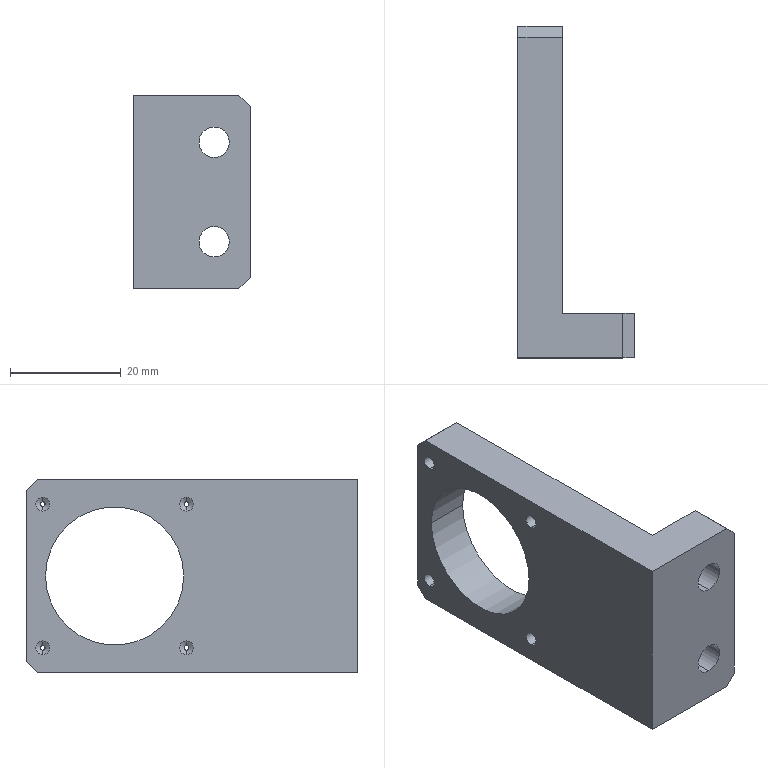Part | NX | features BREP 1 | 1 solid | 34 faces | box 21 x 60 x 35 mm | volume 15917 mm3 | cylinder 14 | plane 12 | cone 8 | commonest cylinder face diameters 2.5 x8 5.5 x4 25 x2
STEP:
#1=CARTESIAN_POINT('',(3.227,27.193,17.5));
#2=VERTEX_POINT('',#1);
#3=CARTESIAN_POINT('',(3.227,2.193,17.5));
#4=VERTEX_POINT('',#3);
#5=CARTESIAN_POINT('',(3.227,14.693,17.5));
#6=DIRECTION('',(-1.,0.,0.));
#7=DIRECTION('',(0.,1.,0.));
#8=AXIS2_PLACEMENT_3D('',#5,#6,#7);
#9=CIRCLE('',#8,12.5);
#10=EDGE_CURVE('',#2,#4,#9,.T.);
#11=ORIENTED_EDGE('',*,*,#10,.T.);
#12=CARTESIAN_POINT('',(11.227,2.193,17.5));
#13=VERTEX_POINT('',#12);
#14=CARTESIAN_POINT('',(3.227,2.193,17.5));
#15=DIRECTION('',(1.,0.,0.));
#16=VECTOR('',#15,1000.);
#17=LINE('',#14,#16);
#18=EDGE_CURVE('',#13,#4,#17,.F.);
#19=ORIENTED_EDGE('',*,*,#18,.F.);
#20=CARTESIAN_POINT('',(11.227,27.193,17.5));
#21=VERTEX_POINT('',#20);
#22=CARTESIAN_POINT('',(11.227,14.693,17.5));
#23=DIRECTION('',(-1.,0.,0.));
#24=DIRECTION('',(0.,1.,0.));
#25=AXIS2_PLACEMENT_3D('',#22,#23,#24);
#26=CIRCLE('',#25,12.5);
#27=EDGE_CURVE('',#21,#13,#26,.T.);
#28=ORIENTED_EDGE('',*,*,#27,.F.);
#29=CARTESIAN_POINT('',(3.227,27.193,17.5));
#30=DIRECTION('',(1.,0.,0.));
#31=VECTOR('',#30,1000.);
#32=LINE('',#29,#31);
#33=EDGE_CURVE('',#21,#2,#32,.F.);
#34=ORIENTED_EDGE('',*,*,#33,.T.);
#35=EDGE_LOOP('',(#11,#19,#28,#34));
#36=FACE_BOUND('',#35,.T.);
#37=CARTESIAN_POINT('',(3.227,14.693,17.5));
#38=DIRECTION('',(1.,0.,0.));
#39=DIRECTION('',(0.,1.,0.));
#40=AXIS2_PLACEMENT_3D('',#37,#38,#39);
#41=CYLINDRICAL_SURFACE('',#40,12.5);
#42=ADVANCED_FACE('',(#36),#41,.F.);
#43=CARTESIAN_POINT('',(10.727,1.693,3.25));
#44=VERTEX_POINT('',#43);
#45=CARTESIAN_POINT('',(10.727,1.693,5.75));
#46=VERTEX_POINT('',#45);
#47=CARTESIAN_POINT('',(10.727,1.693,4.5));
#48=DIRECTION('',(-1.,0.,0.));
#49=DIRECTION('',(0.,0.,1.));
#50=AXIS2_PLACEMENT_3D('',#47,#48,#49);
#51=CIRCLE('',#50,1.25);
#52=EDGE_CURVE('',#44,#46,#51,.T.);
#53=ORIENTED_EDGE('',*,*,#52,.F.);
#54=CARTESIAN_POINT('',(3.227,1.693,3.25));
#55=VERTEX_POINT('',#54);
#56=CARTESIAN_POINT('',(3.227,1.693,3.25));
#57=DIRECTION('',(-1.,0.,0.));
#58=VECTOR('',#57,1000.);
#59=LINE('',#56,#58);
#60=EDGE_CURVE('',#55,#44,#59,.F.);
#61=ORIENTED_EDGE('',*,*,#60,.F.);
#62=CARTESIAN_POINT('',(3.227,1.693,5.75));
#63=VERTEX_POINT('',#62);
#64=CARTESIAN_POINT('',(3.227,1.693,4.5));
#65=DIRECTION('',(-1.,0.,0.));
#66=DIRECTION('',(0.,0.,1.));
#67=AXIS2_PLACEMENT_3D('',#64,#65,#66);
#68=CIRCLE('',#67,1.25);
#69=EDGE_CURVE('',#55,#63,#68,.T.);
#70=ORIENTED_EDGE('',*,*,#69,.T.);
#71=CARTESIAN_POINT('',(3.227,1.693,5.75));
#72=DIRECTION('',(-1.,0.,0.));
#73=VECTOR('',#72,1000.);
#74=LINE('',#71,#73);
#75=EDGE_CURVE('',#63,#46,#74,.F.);
#76=ORIENTED_EDGE('',*,*,#75,.T.);
#77=EDGE_LOOP('',(#53,#61,#70,#76));
#78=FACE_BOUND('',#77,.T.);
#79=CARTESIAN_POINT('',(3.227,1.693,4.5));
#80=DIRECTION('',(-1.,0.,0.));
#81=DIRECTION('',(0.,0.,1.));
#82=AXIS2_PLACEMENT_3D('',#79,#80,#81);
#83=CYLINDRICAL_SURFACE('',#82,1.25);
#84=ADVANCED_FACE('',(#78),#83,.F.);
#85=CARTESIAN_POINT('',(10.727,1.693,29.25));
#86=VERTEX_POINT('',#85);
#87=CARTESIAN_POINT('',(10.727,1.693,31.75));
#88=VERTEX_POINT('',#87);
#89=CARTESIAN_POINT('',(10.727,1.693,30.5));
#90=DIRECTION('',(-1.,0.,0.));
#91=DIRECTION('',(0.,0.,1.));
#92=AXIS2_PLACEMENT_3D('',#89,#90,#91);
#93=CIRCLE('',#92,1.25);
#94=EDGE_CURVE('',#86,#88,#93,.T.);
#95=ORIENTED_EDGE('',*,*,#94,.F.);
#96=CARTESIAN_POINT('',(3.227,1.693,29.25));
#97=VERTEX_POINT('',#96);
#98=CARTESIAN_POINT('',(3.227,1.693,29.25));
#99=DIRECTION('',(-1.,0.,0.));
#100=VECTOR('',#99,1000.);
#101=LINE('',#98,#100);
#102=EDGE_CURVE('',#97,#86,#101,.F.);
#103=ORIENTED_EDGE('',*,*,#102,.F.);
#104=CARTESIAN_POINT('',(3.227,1.693,31.75));
#105=VERTEX_POINT('',#104);
#106=CARTESIAN_POINT('',(3.227,1.693,30.5));
#107=DIRECTION('',(-1.,0.,0.));
#108=DIRECTION('',(0.,0.,1.));
#109=AXIS2_PLACEMENT_3D('',#106,#107,#108);
#110=CIRCLE('',#109,1.25);
#111=EDGE_CURVE('',#97,#105,#110,.T.);
#112=ORIENTED_EDGE('',*,*,#111,.T.);
#113=CARTESIAN_POINT('',(3.227,1.693,31.75));
#114=DIRECTION('',(-1.,0.,0.));
#115=VECTOR('',#114,1000.);
#116=LINE('',#113,#115);
#117=EDGE_CURVE('',#105,#88,#116,.F.);
#118=ORIENTED_EDGE('',*,*,#117,.T.);
#119=EDGE_LOOP('',(#95,#103,#112,#118));
#120=FACE_BOUND('',#119,.T.);
#121=CARTESIAN_POINT('',(3.227,1.693,30.5));
#122=DIRECTION('',(-1.,0.,0.));
#123=DIRECTION('',(0.,0.,1.));
#124=AXIS2_PLACEMENT_3D('',#121,#122,#123);
#125=CYLINDRICAL_SURFACE('',#124,1.25);
#126=ADVANCED_FACE('',(#120),#125,.F.);
#127=CARTESIAN_POINT('',(10.727,27.693,29.25));
#128=VERTEX_POINT('',#127);
#129=CARTESIAN_POINT('',(10.727,27.693,31.75));
#130=VERTEX_POINT('',#129);
#131=CARTESIAN_POINT('',(10.727,27.693,30.5));
#132=DIRECTION('',(-1.,0.,0.));
#133=DIRECTION('',(0.,0.,1.));
#134=AXIS2_PLACEMENT_3D('',#131,#132,#133);
#135=CIRCLE('',#134,1.25);
#136=EDGE_CURVE('',#128,#130,#135,.T.);
#137=ORIENTED_EDGE('',*,*,#136,.F.);
#138=CARTESIAN_POINT('',(3.227,27.693,29.25));
#139=VERTEX_POINT('',#138);
#140=CARTESIAN_POINT('',(3.227,27.693,29.25));
#141=DIRECTION('',(-1.,0.,0.));
#142=VECTOR('',#141,1000.);
#143=LINE('',#140,#142);
#144=EDGE_CURVE('',#139,#128,#143,.F.);
#145=ORIENTED_EDGE('',*,*,#144,.F.);
#146=CARTESIAN_POINT('',(3.227,27.693,31.75));
#147=VERTEX_POINT('',#146);
#148=CARTESIAN_POINT('',(3.227,27.693,30.5));
#149=DIRECTION('',(-1.,0.,0.));
#150=DIRECTION('',(0.,0.,1.));
#151=AXIS2_PLACEMENT_3D('',#148,#149,#150);
#152=CIRCLE('',#151,1.25);
#153=EDGE_CURVE('',#139,#147,#152,.T.);
#154=ORIENTED_EDGE('',*,*,#153,.T.);
#155=CARTESIAN_POINT('',(3.227,27.693,31.75));
#156=DIRECTION('',(-1.,0.,0.));
#157=VECTOR('',#156,1000.);
#158=LINE('',#155,#157);
#159=EDGE_CURVE('',#147,#130,#158,.F.);
#160=ORIENTED_EDGE('',*,*,#159,.T.);
#161=EDGE_LOOP('',(#137,#145,#154,#160));
#162=FACE_BOUND('',#161,.T.);
#163=CARTESIAN_POINT('',(3.227,27.693,30.5));
#164=DIRECTION('',(-1.,0.,0.));
#165=DIRECTION('',(0.,0.,1.));
#166=AXIS2_PLACEMENT_3D('',#163,#164,#165);
#167=CYLINDRICAL_SURFACE('',#166,1.25);
#168=ADVANCED_FACE('',(#162),#167,.F.);
#169=CARTESIAN_POINT('',(10.727,27.693,3.25));
#170=VERTEX_POINT('',#169);
#171=CARTESIAN_POINT('',(10.727,27.693,5.75));
#172=VERTEX_POINT('',#171);
#173=CARTESIAN_POINT('',(10.727,27.693,4.5));
#174=DIRECTION('',(-1.,0.,0.));
#175=DIRECTION('',(0.,0.,1.));
#176=AXIS2_PLACEMENT_3D('',#173,#174,#175);
#177=CIRCLE('',#176,1.25);
#178=EDGE_CURVE('',#170,#172,#177,.T.);
#179=ORIENTED_EDGE('',*,*,#178,.F.);
#180=CARTESIAN_POINT('',(3.227,27.693,3.25));
#181=VERTEX_POINT('',#180);
#182=CARTESIAN_POINT('',(3.227,27.693,3.25));
#183=DIRECTION('',(-1.,0.,0.));
#184=VECTOR('',#183,1000.);
#185=LINE('',#182,#184);
#186=EDGE_CURVE('',#181,#170,#185,.F.);
#187=ORIENTED_EDGE('',*,*,#186,.F.);
#188=CARTESIAN_POINT('',(3.227,27.693,5.75));
#189=VERTEX_POINT('',#188);
#190=CARTESIAN_POINT('',(3.227,27.693,4.5));
#191=DIRECTION('',(-1.,0.,0.));
#192=DIRECTION('',(0.,0.,1.));
#193=AXIS2_PLACEMENT_3D('',#190,#191,#192);
#194=CIRCLE('',#193,1.25);
#195=EDGE_CURVE('',#181,#189,#194,.T.);
#196=ORIENTED_EDGE('',*,*,#195,.T.);
#197=CARTESIAN_POINT('',(3.227,27.693,5.75));
#198=DIRECTION('',(-1.,0.,0.));
#199=VECTOR('',#198,1000.);
#200=LINE('',#197,#199);
#201=EDGE_CURVE('',#189,#172,#200,.F.);
#202=ORIENTED_EDGE('',*,*,#201,.T.);
#203=EDGE_LOOP('',(#179,#187,#196,#202));
#204=FACE_BOUND('',#203,.T.);
#205=CARTESIAN_POINT('',(3.227,27.693,4.5));
#206=DIRECTION('',(-1.,0.,0.));
#207=DIRECTION('',(0.,0.,1.));
#208=AXIS2_PLACEMENT_3D('',#205,#206,#207);
#209=CYLINDRICAL_SURFACE('',#208,1.25);
#210=ADVANCED_FACE('',(#204),#209,.F.);
#211=CARTESIAN_POINT('',(17.727,-29.307,29.25));
#212=VERTEX_POINT('',#211);
#213=CARTESIAN_POINT('',(17.727,-29.307,23.75));
#214=VERTEX_POINT('',#213);
#215=CARTESIAN_POINT('',(17.727,-29.307,26.5));
#216=DIRECTION('',(0.,-1.,0.));
#217=DIRECTION('',(0.,0.,1.));
#218=AXIS2_PLACEMENT_3D('',#215,#216,#217);
#219=CIRCLE('',#218,2.75);
#220=EDGE_CURVE('',#212,#214,#219,.T.);
#221=ORIENTED_EDGE('',*,*,#220,.T.);
#222=CARTESIAN_POINT('',(17.727,-21.307,23.75));
#223=VERTEX_POINT('',#222);
#224=CARTESIAN_POINT('',(17.727,-29.307,23.75));
#225=DIRECTION('',(0.,1.,0.));
#226=VECTOR('',#225,1000.);
#227=LINE('',#224,#226);
#228=EDGE_CURVE('',#223,#214,#227,.F.);
#229=ORIENTED_EDGE('',*,*,#228,.F.);
#230=CARTESIAN_POINT('',(17.727,-21.307,29.25));
#231=VERTEX_POINT('',#230);
#232=CARTESIAN_POINT('',(17.727,-21.307,26.5));
#233=DIRECTION('',(0.,1.,0.));
#234=DIRECTION('',(0.,0.,1.));
#235=AXIS2_PLACEMENT_3D('',#232,#233,#234);
#236=CIRCLE('',#235,2.75);
#237=EDGE_CURVE('',#223,#231,#236,.T.);
#238=ORIENTED_EDGE('',*,*,#237,.T.);
#239=CARTESIAN_POINT('',(17.727,-29.307,29.25));
#240=DIRECTION('',(0.,1.,0.));
#241=VECTOR('',#240,1000.);
#242=LINE('',#239,#241);
#243=EDGE_CURVE('',#231,#212,#242,.F.);
#244=ORIENTED_EDGE('',*,*,#243,.T.);
#245=EDGE_LOOP('',(#221,#229,#238,#244));
#246=FACE_BOUND('',#245,.T.);
#247=CARTESIAN_POINT('',(17.727,-29.307,26.5));
#248=DIRECTION('',(0.,1.,0.));
#249=DIRECTION('',(0.,0.,1.));
#250=AXIS2_PLACEMENT_3D('',#247,#248,#249);
#251=CYLINDRICAL_SURFACE('',#250,2.75);
#252=ADVANCED_FACE('',(#246),#251,.F.);
#253=CARTESIAN_POINT('',(17.727,-29.307,11.25));
#254=VERTEX_POINT('',#253);
#255=CARTESIAN_POINT('',(17.727,-29.307,5.75));
#256=VERTEX_POINT('',#255);
#257=CARTESIAN_POINT('',(17.727,-29.307,8.5));
#258=DIRECTION('',(0.,-1.,0.));
#259=DIRECTION('',(0.,0.,1.));
#260=AXIS2_PLACEMENT_3D('',#257,#258,#259);
#261=CIRCLE('',#260,2.75);
#262=EDGE_CURVE('',#254,#256,#261,.T.);
#263=ORIENTED_EDGE('',*,*,#262,.T.);
#264=CARTESIAN_POINT('',(17.727,-21.307,5.75));
#265=VERTEX_POINT('',#264);
#266=CARTESIAN_POINT('',(17.727,-29.307,5.75));
#267=DIRECTION('',(0.,1.,0.));
#268=VECTOR('',#267,1000.);
#269=LINE('',#266,#268);
#270=EDGE_CURVE('',#265,#256,#269,.F.);
#271=ORIENTED_EDGE('',*,*,#270,.F.);
#272=CARTESIAN_POINT('',(17.727,-21.307,11.25));
#273=VERTEX_POINT('',#272);
#274=CARTESIAN_POINT('',(17.727,-21.307,8.5));
#275=DIRECTION('',(0.,1.,0.));
#276=DIRECTION('',(0.,0.,1.));
#277=AXIS2_PLACEMENT_3D('',#274,#275,#276);
#278=CIRCLE('',#277,2.75);
#279=EDGE_CURVE('',#265,#273,#278,.T.);
#280=ORIENTED_EDGE('',*,*,#279,.T.);
#281=CARTESIAN_POINT('',(17.727,-29.307,11.25));
#282=DIRECTION('',(0.,1.,0.));
#283=VECTOR('',#282,1000.);
#284=LINE('',#281,#283);
#285=EDGE_CURVE('',#273,#254,#284,.F.);
#286=ORIENTED_EDGE('',*,*,#285,.T.);
#287=EDGE_LOOP('',(#263,#271,#280,#286));
#288=FACE_BOUND('',#287,.T.);
#289=CARTESIAN_POINT('',(17.727,-29.307,8.5));
#290=DIRECTION('',(0.,1.,0.));
#291=DIRECTION('',(0.,0.,1.));
#292=AXIS2_PLACEMENT_3D('',#289,#290,#291);
#293=CYLINDRICAL_SURFACE('',#292,2.75);
#294=ADVANCED_FACE('',(#288),#293,.F.);
#295=CARTESIAN_POINT('',(11.227,1.693,4.918));
#296=VERTEX_POINT('',#295);
#297=CARTESIAN_POINT('',(11.227,1.693,4.082));
#298=VERTEX_POINT('',#297);
#299=CARTESIAN_POINT('',(11.227,1.693,4.5));
#300=DIRECTION('',(1.,0.,0.));
#301=DIRECTION('',(0.,0.,1.));
#302=AXIS2_PLACEMENT_3D('',#299,#300,#301);
#303=CIRCLE('',#302,0.4179);
#304=EDGE_CURVE('',#296,#298,#303,.T.);
#305=ORIENTED_EDGE('',*,*,#304,.T.);
#306=CARTESIAN_POINT('',(10.727,1.693,3.25));
#307=DIRECTION('',(-0.515,0.,-0.8572));
#308=VECTOR('',#307,1000.);
#309=LINE('',#306,#308);
#310=EDGE_CURVE('',#44,#298,#309,.F.);
#311=ORIENTED_EDGE('',*,*,#310,.F.);
#312=ORIENTED_EDGE('',*,*,#52,.T.);
#313=CARTESIAN_POINT('',(10.727,1.693,5.75));
#314=DIRECTION('',(-0.515,0.,0.8572));
#315=VECTOR('',#314,1000.);
#316=LINE('',#313,#315);
#317=EDGE_CURVE('',#46,#296,#316,.F.);
#318=ORIENTED_EDGE('',*,*,#317,.T.);
#319=EDGE_LOOP('',(#305,#311,#312,#318));
#320=FACE_BOUND('',#319,.T.);
#321=CARTESIAN_POINT('',(10.727,1.693,4.5));
#322=DIRECTION('',(-1.,0.,0.));
#323=DIRECTION('',(0.,0.,1.));
#324=AXIS2_PLACEMENT_3D('',#321,#322,#323);
#325=CONICAL_SURFACE('',#324,1.25,1.03);
#326=ADVANCED_FACE('',(#320),#325,.F.);
#327=CARTESIAN_POINT('',(11.227,1.693,30.918));
#328=VERTEX_POINT('',#327);
#329=CARTESIAN_POINT('',(11.227,1.693,30.082));
#330=VERTEX_POINT('',#329);
#331=CARTESIAN_POINT('',(11.227,1.693,30.5));
#332=DIRECTION('',(1.,0.,0.));
#333=DIRECTION('',(0.,0.,1.));
#334=AXIS2_PLACEMENT_3D('',#331,#332,#333);
#335=CIRCLE('',#334,0.4179);
#336=EDGE_CURVE('',#328,#330,#335,.T.);
#337=ORIENTED_EDGE('',*,*,#336,.T.);
#338=CARTESIAN_POINT('',(10.727,1.693,29.25));
#339=DIRECTION('',(-0.515,0.,-0.8572));
#340=VECTOR('',#339,1000.);
#341=LINE('',#338,#340);
#342=EDGE_CURVE('',#86,#330,#341,.F.);
#343=ORIENTED_EDGE('',*,*,#342,.F.);
#344=ORIENTED_EDGE('',*,*,#94,.T.);
#345=CARTESIAN_POINT('',(10.727,1.693,31.75));
#346=DIRECTION('',(-0.515,0.,0.8572));
#347=VECTOR('',#346,1000.);
#348=LINE('',#345,#347);
#349=EDGE_CURVE('',#88,#328,#348,.F.);
#350=ORIENTED_EDGE('',*,*,#349,.T.);
#351=EDGE_LOOP('',(#337,#343,#344,#350));
#352=FACE_BOUND('',#351,.T.);
#353=CARTESIAN_POINT('',(10.727,1.693,30.5));
#354=DIRECTION('',(-1.,0.,0.));
#355=DIRECTION('',(0.,0.,1.));
#356=AXIS2_PLACEMENT_3D('',#353,#354,#355);
#357=CONICAL_SURFACE('',#356,1.25,1.03);
#358=ADVANCED_FACE('',(#352),#357,.F.);
#359=CARTESIAN_POINT('',(11.227,27.693,30.918));
#360=VERTEX_POINT('',#359);
#361=CARTESIAN_POINT('',(11.227,27.693,30.082));
#362=VERTEX_POINT('',#361);
#363=CARTESIAN_POINT('',(11.227,27.693,30.5));
#364=DIRECTION('',(1.,0.,0.));
#365=DIRECTION('',(0.,0.,1.));
#366=AXIS2_PLACEMENT_3D('',#363,#364,#365);
#367=CIRCLE('',#366,0.4179);
#368=EDGE_CURVE('',#360,#362,#367,.T.);
#369=ORIENTED_EDGE('',*,*,#368,.T.);
#370=CARTESIAN_POINT('',(10.727,27.693,29.25));
#371=DIRECTION('',(-0.515,0.,-0.8572));
#372=VECTOR('',#371,1000.);
#373=LINE('',#370,#372);
#374=EDGE_CURVE('',#128,#362,#373,.F.);
#375=ORIENTED_EDGE('',*,*,#374,.F.);
#376=ORIENTED_EDGE('',*,*,#136,.T.);
#377=CARTESIAN_POINT('',(10.727,27.693,31.75));
#378=DIRECTION('',(-0.515,0.,0.8572));
#379=VECTOR('',#378,1000.);
#380=LINE('',#377,#379);
#381=EDGE_CURVE('',#130,#360,#380,.F.);
#382=ORIENTED_EDGE('',*,*,#381,.T.);
#383=EDGE_LOOP('',(#369,#375,#376,#382));
#384=FACE_BOUND('',#383,.T.);
#385=CARTESIAN_POINT('',(10.727,27.693,30.5));
#386=DIRECTION('',(-1.,0.,0.));
#387=DIRECTION('',(0.,0.,1.));
#388=AXIS2_PLACEMENT_3D('',#385,#386,#387);
#389=CONICAL_SURFACE('',#388,1.25,1.03);
#390=ADVANCED_FACE('',(#384),#389,.F.);
#391=CARTESIAN_POINT('',(11.227,27.693,4.918));
#392=VERTEX_POINT('',#391);
#393=CARTESIAN_POINT('',(11.227,27.693,4.082));
#394=VERTEX_POINT('',#393);
#395=CARTESIAN_POINT('',(11.227,27.693,4.5));
#396=DIRECTION('',(1.,0.,0.));
#397=DIRECTION('',(0.,0.,1.));
#398=AXIS2_PLACEMENT_3D('',#395,#396,#397);
#399=CIRCLE('',#398,0.4179);
#400=EDGE_CURVE('',#392,#394,#399,.T.);
#401=ORIENTED_EDGE('',*,*,#400,.T.);
#402=CARTESIAN_POINT('',(10.727,27.693,3.25));
#403=DIRECTION('',(-0.515,0.,-0.8572));
#404=VECTOR('',#403,1000.);
#405=LINE('',#402,#404);
#406=EDGE_CURVE('',#170,#394,#405,.F.);
#407=ORIENTED_EDGE('',*,*,#406,.F.);
#408=ORIENTED_EDGE('',*,*,#178,.T.);
#409=CARTESIAN_POINT('',(10.727,27.693,5.75));
#410=DIRECTION('',(-0.515,0.,0.8572));
#411=VECTOR('',#410,1000.);
#412=LINE('',#409,#411);
#413=EDGE_CURVE('',#172,#392,#412,.F.);
#414=ORIENTED_EDGE('',*,*,#413,.T.);
#415=EDGE_LOOP('',(#401,#407,#408,#414));
#416=FACE_BOUND('',#415,.T.);
#417=CARTESIAN_POINT('',(10.727,27.693,4.5));
#418=DIRECTION('',(-1.,0.,0.));
#419=DIRECTION('',(0.,0.,1.));
#420=AXIS2_PLACEMENT_3D('',#417,#418,#419);
#421=CONICAL_SURFACE('',#420,1.25,1.03);
#422=ADVANCED_FACE('',(#416),#421,.F.);
#423=CARTESIAN_POINT('',(3.227,28.693,0.));
#424=VERTEX_POINT('',#423);
#425=CARTESIAN_POINT('',(3.227,30.693,2.));
#426=VERTEX_POINT('',#425);
#427=CARTESIAN_POINT('',(3.227,28.693,0.));
#428=DIRECTION('',(0.,0.7071,0.7071));
#429=VECTOR('',#428,1000.);
#430=LINE('',#427,#429);
#431=EDGE_CURVE('',#424,#426,#430,.T.);
#432=ORIENTED_EDGE('',*,*,#431,.F.);
#433=CARTESIAN_POINT('',(3.227,-29.307,0.));
#434=VERTEX_POINT('',#433);
#435=CARTESIAN_POINT('',(3.227,-20.189,0.));
#436=DIRECTION('',(0.,1.,0.));
#437=VECTOR('',#436,1000.);
#438=LINE('',#435,#437);
#439=EDGE_CURVE('',#434,#424,#438,.T.);
#440=ORIENTED_EDGE('',*,*,#439,.F.);
#441=CARTESIAN_POINT('',(3.227,-29.307,35.));
#442=VERTEX_POINT('',#441);
#443=CARTESIAN_POINT('',(3.227,-29.307,35.));
#444=DIRECTION('',(0.,0.,-1.));
#445=VECTOR('',#444,1000.);
#446=LINE('',#443,#445);
#447=EDGE_CURVE('',#442,#434,#446,.T.);
#448=ORIENTED_EDGE('',*,*,#447,.F.);
#449=CARTESIAN_POINT('',(3.227,28.693,35.));
#450=VERTEX_POINT('',#449);
#451=CARTESIAN_POINT('',(3.227,-20.189,35.));
#452=DIRECTION('',(0.,-1.,0.));
#453=VECTOR('',#452,1000.);
#454=LINE('',#451,#453);
#455=EDGE_CURVE('',#450,#442,#454,.T.);
#456=ORIENTED_EDGE('',*,*,#455,.F.);
#457=CARTESIAN_POINT('',(3.227,30.693,33.));
#458=VERTEX_POINT('',#457);
#459=CARTESIAN_POINT('',(3.227,30.693,33.));
#460=DIRECTION('',(0.,-0.7071,0.7071));
#461=VECTOR('',#460,1000.);
#462=LINE('',#459,#461);
#463=EDGE_CURVE('',#458,#450,#462,.T.);
#464=ORIENTED_EDGE('',*,*,#463,.F.);
#465=CARTESIAN_POINT('',(3.227,30.693,35.));
#466=DIRECTION('',(0.,0.,1.));
#467=VECTOR('',#466,1000.);
#468=LINE('',#465,#467);
#469=EDGE_CURVE('',#426,#458,#468,.T.);
#470=ORIENTED_EDGE('',*,*,#469,.F.);
#471=EDGE_LOOP('',(#432,#440,#448,#456,#464,#470));
#472=FACE_BOUND('',#471,.T.);
#473=ORIENTED_EDGE('',*,*,#10,.F.);
#474=CARTESIAN_POINT('',(3.227,14.693,17.5));
#475=DIRECTION('',(-1.,0.,0.));
#476=DIRECTION('',(0.,1.,0.));
#477=AXIS2_PLACEMENT_3D('',#474,#475,#476);
#478=CIRCLE('',#477,12.5);
#479=EDGE_CURVE('',#4,#2,#478,.T.);
#480=ORIENTED_EDGE('',*,*,#479,.F.);
#481=EDGE_LOOP('',(#473,#480));
#482=FACE_BOUND('',#481,.T.);
#483=CARTESIAN_POINT('',(3.227,1.693,4.5));
#484=DIRECTION('',(-1.,0.,0.));
#485=DIRECTION('',(0.,0.,1.));
#486=AXIS2_PLACEMENT_3D('',#483,#484,#485);
#487=CIRCLE('',#486,1.25);
#488=EDGE_CURVE('',#63,#55,#487,.T.);
#489=ORIENTED_EDGE('',*,*,#488,.F.);
#490=ORIENTED_EDGE('',*,*,#69,.F.);
#491=EDGE_LOOP('',(#489,#490));
#492=FACE_BOUND('',#491,.T.);
#493=CARTESIAN_POINT('',(3.227,1.693,30.5));
#494=DIRECTION('',(-1.,0.,0.));
#495=DIRECTION('',(0.,0.,1.));
#496=AXIS2_PLACEMENT_3D('',#493,#494,#495);
#497=CIRCLE('',#496,1.25);
#498=EDGE_CURVE('',#105,#97,#497,.T.);
#499=ORIENTED_EDGE('',*,*,#498,.F.);
#500=ORIENTED_EDGE('',*,*,#111,.F.);
#501=EDGE_LOOP('',(#499,#500));
#502=FACE_BOUND('',#501,.T.);
#503=CARTESIAN_POINT('',(3.227,27.693,30.5));
#504=DIRECTION('',(-1.,0.,0.));
#505=DIRECTION('',(0.,0.,1.));
#506=AXIS2_PLACEMENT_3D('',#503,#504,#505);
#507=CIRCLE('',#506,1.25);
#508=EDGE_CURVE('',#147,#139,#507,.T.);
#509=ORIENTED_EDGE('',*,*,#508,.F.);
#510=ORIENTED_EDGE('',*,*,#153,.F.);
#511=EDGE_LOOP('',(#509,#510));
#512=FACE_BOUND('',#511,.T.);
#513=CARTESIAN_POINT('',(3.227,27.693,4.5));
#514=DIRECTION('',(-1.,0.,0.));
#515=DIRECTION('',(0.,0.,1.));
#516=AXIS2_PLACEMENT_3D('',#513,#514,#515);
#517=CIRCLE('',#516,1.25);
#518=EDGE_CURVE('',#189,#181,#517,.T.);
#519=ORIENTED_EDGE('',*,*,#518,.F.);
#520=ORIENTED_EDGE('',*,*,#195,.F.);
#521=EDGE_LOOP('',(#519,#520));
#522=FACE_BOUND('',#521,.T.);
#523=CARTESIAN_POINT('',(3.227,-20.189,35.));
#524=DIRECTION('',(1.,0.,0.));
#525=DIRECTION('',(0.,1.,0.));
#526=AXIS2_PLACEMENT_3D('',#523,#524,#525);
#527=PLANE('',#526);
#528=ADVANCED_FACE('',(#472,#482,#492,#502,#512,#522),#527,.F.);
#529=CARTESIAN_POINT('',(11.227,30.693,2.));
#530=VERTEX_POINT('',#529);
#531=CARTESIAN_POINT('',(11.227,30.693,2.));
#532=DIRECTION('',(1.,0.,0.));
#533=VECTOR('',#532,1000.);
#534=LINE('',#531,#533);
#535=EDGE_CURVE('',#426,#530,#534,.T.);
#536=ORIENTED_EDGE('',*,*,#535,.F.);
#537=ORIENTED_EDGE('',*,*,#469,.T.);
#538=CARTESIAN_POINT('',(11.227,30.693,33.));
#539=VERTEX_POINT('',#538);
#540=CARTESIAN_POINT('',(11.227,30.693,33.));
#541=DIRECTION('',(-1.,0.,0.));
#542=VECTOR('',#541,1000.);
#543=LINE('',#540,#542);
#544=EDGE_CURVE('',#539,#458,#543,.T.);
#545=ORIENTED_EDGE('',*,*,#544,.F.);
#546=CARTESIAN_POINT('',(11.227,30.693,35.));
#547=DIRECTION('',(0.,0.,1.));
#548=VECTOR('',#547,1000.);
#549=LINE('',#546,#548);
#550=EDGE_CURVE('',#530,#539,#549,.T.);
#551=ORIENTED_EDGE('',*,*,#550,.F.);
#552=EDGE_LOOP('',(#536,#537,#545,#551));
#553=FACE_BOUND('',#552,.T.);
#554=CARTESIAN_POINT('',(11.227,30.693,35.));
#555=DIRECTION('',(0.,-1.,0.));
#556=DIRECTION('',(0.,0.,-1.));
#557=AXIS2_PLACEMENT_3D('',#554,#555,#556);
#558=PLANE('',#557);
#559=ADVANCED_FACE('',(#553),#558,.F.);
#560=CARTESIAN_POINT('',(11.227,28.693,0.));
#561=VERTEX_POINT('',#560);
#562=CARTESIAN_POINT('',(11.227,28.693,0.));
#563=DIRECTION('',(1.,0.,0.));
#564=VECTOR('',#563,1000.);
#565=LINE('',#562,#564);
#566=EDGE_CURVE('',#424,#561,#565,.T.);
#567=ORIENTED_EDGE('',*,*,#566,.F.);
#568=ORIENTED_EDGE('',*,*,#431,.T.);
#569=ORIENTED_EDGE('',*,*,#535,.T.);
#570=CARTESIAN_POINT('',(11.227,30.693,2.));
#571=DIRECTION('',(0.,0.7071,0.7071));
#572=VECTOR('',#571,1000.);
#573=LINE('',#570,#572);
#574=EDGE_CURVE('',#561,#530,#573,.T.);
#575=ORIENTED_EDGE('',*,*,#574,.F.);
#576=EDGE_LOOP('',(#567,#568,#569,#575));
#577=FACE_BOUND('',#576,.T.);
#578=CARTESIAN_POINT('',(11.227,30.693,2.));
#579=DIRECTION('',(0.,-0.7071,0.7071));
#580=DIRECTION('',(-1.,0.,0.));
#581=AXIS2_PLACEMENT_3D('',#578,#579,#580);
#582=PLANE('',#581);
#583=ADVANCED_FACE('',(#577),#582,.F.);
#584=ORIENTED_EDGE('',*,*,#566,.T.);
#585=CARTESIAN_POINT('',(11.227,-21.307,0.));
#586=VERTEX_POINT('',#585);
#587=CARTESIAN_POINT('',(11.227,-21.307,0.));
#588=DIRECTION('',(0.,1.,0.));
#589=VECTOR('',#588,1000.);
#590=LINE('',#587,#589);
#591=EDGE_CURVE('',#586,#561,#590,.T.);
#592=ORIENTED_EDGE('',*,*,#591,.F.);
#593=CARTESIAN_POINT('',(22.227,-21.307,0.));
#594=VERTEX_POINT('',#593);
#595=CARTESIAN_POINT('',(11.227,-21.307,0.));
#596=DIRECTION('',(-1.,0.,0.));
#597=VECTOR('',#596,1000.);
#598=LINE('',#595,#597);
#599=EDGE_CURVE('',#594,#586,#598,.T.);
#600=ORIENTED_EDGE('',*,*,#599,.F.);
#601=CARTESIAN_POINT('',(22.227,-29.307,0.));
#602=VERTEX_POINT('',#601);
#603=CARTESIAN_POINT('',(22.227,-21.307,0.));
#604=DIRECTION('',(0.,1.,0.));
#605=VECTOR('',#604,1000.);
#606=LINE('',#603,#605);
#607=EDGE_CURVE('',#602,#594,#606,.T.);
#608=ORIENTED_EDGE('',*,*,#607,.F.);
#609=CARTESIAN_POINT('',(11.227,-29.307,0.));
#610=DIRECTION('',(1.,0.,0.));
#611=VECTOR('',#610,1000.);
#612=LINE('',#609,#611);
#613=EDGE_CURVE('',#434,#602,#612,.T.);
#614=ORIENTED_EDGE('',*,*,#613,.F.);
#615=ORIENTED_EDGE('',*,*,#439,.T.);
#616=EDGE_LOOP('',(#584,#592,#600,#608,#614,#615));
#617=FACE_BOUND('',#616,.T.);
#618=CARTESIAN_POINT('',(11.227,-21.307,0.));
#619=DIRECTION('',(0.,0.,1.));
#620=DIRECTION('',(1.,0.,0.));
#621=AXIS2_PLACEMENT_3D('',#618,#619,#620);
#622=PLANE('',#621);
#623=ADVANCED_FACE('',(#617),#622,.F.);
#624=CARTESIAN_POINT('',(22.227,-29.307,35.));
#625=VERTEX_POINT('',#624);
#626=CARTESIAN_POINT('',(24.227,-29.307,33.));
#627=VERTEX_POINT('',#626);
#628=CARTESIAN_POINT('',(22.227,-29.307,35.));
#629=DIRECTION('',(0.7071,0.,-0.7071));
#630=VECTOR('',#629,1000.);
#631=LINE('',#628,#630);
#632=EDGE_CURVE('',#625,#627,#631,.T.);
#633=ORIENTED_EDGE('',*,*,#632,.F.);
#634=CARTESIAN_POINT('',(3.227,-29.307,35.));
#635=DIRECTION('',(1.,0.,0.));
#636=VECTOR('',#635,1000.);
#637=LINE('',#634,#636);
#638=EDGE_CURVE('',#442,#625,#637,.T.);
#639=ORIENTED_EDGE('',*,*,#638,.F.);
#640=ORIENTED_EDGE('',*,*,#447,.T.);
#641=ORIENTED_EDGE('',*,*,#613,.T.);
#642=CARTESIAN_POINT('',(24.227,-29.307,2.));
#643=VERTEX_POINT('',#642);
#644=CARTESIAN_POINT('',(24.227,-29.307,2.));
#645=DIRECTION('',(-0.7071,0.,-0.7071));
#646=VECTOR('',#645,1000.);
#647=LINE('',#644,#646);
#648=EDGE_CURVE('',#643,#602,#647,.T.);
#649=ORIENTED_EDGE('',*,*,#648,.F.);
#650=CARTESIAN_POINT('',(24.227,-29.307,35.));
#651=DIRECTION('',(0.,0.,-1.));
#652=VECTOR('',#651,1000.);
#653=LINE('',#650,#652);
#654=EDGE_CURVE('',#627,#643,#653,.T.);
#655=ORIENTED_EDGE('',*,*,#654,.F.);
#656=EDGE_LOOP('',(#633,#639,#640,#641,#649,#655));
#657=FACE_BOUND('',#656,.T.);
#658=ORIENTED_EDGE('',*,*,#220,.F.);
#659=CARTESIAN_POINT('',(17.727,-29.307,26.5));
#660=DIRECTION('',(0.,-1.,0.));
#661=DIRECTION('',(0.,0.,1.));
#662=AXIS2_PLACEMENT_3D('',#659,#660,#661);
#663=CIRCLE('',#662,2.75);
#664=EDGE_CURVE('',#214,#212,#663,.T.);
#665=ORIENTED_EDGE('',*,*,#664,.F.);
#666=EDGE_LOOP('',(#658,#665));
#667=FACE_BOUND('',#666,.T.);
#668=ORIENTED_EDGE('',*,*,#262,.F.);
#669=CARTESIAN_POINT('',(17.727,-29.307,8.5));
#670=DIRECTION('',(0.,-1.,0.));
#671=DIRECTION('',(0.,0.,1.));
#672=AXIS2_PLACEMENT_3D('',#669,#670,#671);
#673=CIRCLE('',#672,2.75);
#674=EDGE_CURVE('',#256,#254,#673,.T.);
#675=ORIENTED_EDGE('',*,*,#674,.F.);
#676=EDGE_LOOP('',(#668,#675));
#677=FACE_BOUND('',#676,.T.);
#678=CARTESIAN_POINT('',(3.227,-29.307,35.));
#679=DIRECTION('',(0.,1.,0.));
#680=DIRECTION('',(1.,0.,0.));
#681=AXIS2_PLACEMENT_3D('',#678,#679,#680);
#682=PLANE('',#681);
#683=ADVANCED_FACE('',(#657,#667,#677),#682,.F.);
#684=CARTESIAN_POINT('',(22.227,-21.307,35.));
#685=VERTEX_POINT('',#684);
#686=CARTESIAN_POINT('',(22.227,-21.307,35.));
#687=DIRECTION('',(0.,1.,0.));
#688=VECTOR('',#687,1000.);
#689=LINE('',#686,#688);
#690=EDGE_CURVE('',#625,#685,#689,.T.);
#691=ORIENTED_EDGE('',*,*,#690,.T.);
#692=CARTESIAN_POINT('',(11.227,-21.307,35.));
#693=VERTEX_POINT('',#692);
#694=CARTESIAN_POINT('',(11.227,-21.307,35.));
#695=DIRECTION('',(-1.,0.,0.));
#696=VECTOR('',#695,1000.);
#697=LINE('',#694,#696);
#698=EDGE_CURVE('',#685,#693,#697,.T.);
#699=ORIENTED_EDGE('',*,*,#698,.T.);
#700=CARTESIAN_POINT('',(11.227,28.693,35.));
#701=VERTEX_POINT('',#700);
#702=CARTESIAN_POINT('',(11.227,-21.307,35.));
#703=DIRECTION('',(0.,1.,0.));
#704=VECTOR('',#703,1000.);
#705=LINE('',#702,#704);
#706=EDGE_CURVE('',#693,#701,#705,.T.);
#707=ORIENTED_EDGE('',*,*,#706,.T.);
#708=CARTESIAN_POINT('',(11.227,28.693,35.));
#709=DIRECTION('',(-1.,0.,0.));
#710=VECTOR('',#709,1000.);
#711=LINE('',#708,#710);
#712=EDGE_CURVE('',#701,#450,#711,.T.);
#713=ORIENTED_EDGE('',*,*,#712,.T.);
#714=ORIENTED_EDGE('',*,*,#455,.T.);
#715=ORIENTED_EDGE('',*,*,#638,.T.);
#716=EDGE_LOOP('',(#691,#699,#707,#713,#714,#715));
#717=FACE_BOUND('',#716,.T.);
#718=CARTESIAN_POINT('',(11.227,-21.307,35.));
#719=DIRECTION('',(0.,0.,1.));
#720=DIRECTION('',(1.,0.,0.));
#721=AXIS2_PLACEMENT_3D('',#718,#719,#720);
#722=PLANE('',#721);
#723=ADVANCED_FACE('',(#717),#722,.T.);
#724=ORIENTED_EDGE('',*,*,#463,.T.);
#725=ORIENTED_EDGE('',*,*,#712,.F.);
#726=CARTESIAN_POINT('',(11.227,28.693,35.));
#727=DIRECTION('',(0.,0.7071,-0.7071));
#728=VECTOR('',#727,1000.);
#729=LINE('',#726,#728);
#730=EDGE_CURVE('',#701,#539,#729,.T.);
#731=ORIENTED_EDGE('',*,*,#730,.T.);
#732=ORIENTED_EDGE('',*,*,#544,.T.);
#733=EDGE_LOOP('',(#724,#725,#731,#732));
#734=FACE_BOUND('',#733,.T.);
#735=CARTESIAN_POINT('',(11.227,28.693,35.));
#736=DIRECTION('',(0.,0.7071,0.7071));
#737=DIRECTION('',(1.,0.,0.));
#738=AXIS2_PLACEMENT_3D('',#735,#736,#737);
#739=PLANE('',#738);
#740=ADVANCED_FACE('',(#734),#739,.T.);
#741=ORIENTED_EDGE('',*,*,#18,.T.);
#742=ORIENTED_EDGE('',*,*,#479,.T.);
#743=ORIENTED_EDGE('',*,*,#33,.F.);
#744=CARTESIAN_POINT('',(11.227,14.693,17.5));
#745=DIRECTION('',(-1.,0.,0.));
#746=DIRECTION('',(0.,1.,0.));
#747=AXIS2_PLACEMENT_3D('',#744,#745,#746);
#748=CIRCLE('',#747,12.5);
#749=EDGE_CURVE('',#13,#21,#748,.T.);
#750=ORIENTED_EDGE('',*,*,#749,.F.);
#751=EDGE_LOOP('',(#741,#742,#743,#750));
#752=FACE_BOUND('',#751,.T.);
#753=CARTESIAN_POINT('',(3.227,14.693,17.5));
#754=DIRECTION('',(1.,0.,0.));
#755=DIRECTION('',(0.,1.,0.));
#756=AXIS2_PLACEMENT_3D('',#753,#754,#755);
#757=CYLINDRICAL_SURFACE('',#756,12.5);
#758=ADVANCED_FACE('',(#752),#757,.F.);
#759=ORIENTED_EDGE('',*,*,#60,.T.);
#760=CARTESIAN_POINT('',(10.727,1.693,4.5));
#761=DIRECTION('',(-1.,0.,0.));
#762=DIRECTION('',(0.,0.,1.));
#763=AXIS2_PLACEMENT_3D('',#760,#761,#762);
#764=CIRCLE('',#763,1.25);
#765=EDGE_CURVE('',#46,#44,#764,.T.);
#766=ORIENTED_EDGE('',*,*,#765,.F.);
#767=ORIENTED_EDGE('',*,*,#75,.F.);
#768=ORIENTED_EDGE('',*,*,#488,.T.);
#769=EDGE_LOOP('',(#759,#766,#767,#768));
#770=FACE_BOUND('',#769,.T.);
#771=CARTESIAN_POINT('',(3.227,1.693,4.5));
#772=DIRECTION('',(-1.,0.,0.));
#773=DIRECTION('',(0.,0.,1.));
#774=AXIS2_PLACEMENT_3D('',#771,#772,#773);
#775=CYLINDRICAL_SURFACE('',#774,1.25);
#776=ADVANCED_FACE('',(#770),#775,.F.);
#777=ORIENTED_EDGE('',*,*,#102,.T.);
#778=CARTESIAN_POINT('',(10.727,1.693,30.5));
#779=DIRECTION('',(-1.,0.,0.));
#780=DIRECTION('',(0.,0.,1.));
#781=AXIS2_PLACEMENT_3D('',#778,#779,#780);
#782=CIRCLE('',#781,1.25);
#783=EDGE_CURVE('',#88,#86,#782,.T.);
#784=ORIENTED_EDGE('',*,*,#783,.F.);
#785=ORIENTED_EDGE('',*,*,#117,.F.);
#786=ORIENTED_EDGE('',*,*,#498,.T.);
#787=EDGE_LOOP('',(#777,#784,#785,#786));
#788=FACE_BOUND('',#787,.T.);
#789=CARTESIAN_POINT('',(3.227,1.693,30.5));
#790=DIRECTION('',(-1.,0.,0.));
#791=DIRECTION('',(0.,0.,1.));
#792=AXIS2_PLACEMENT_3D('',#789,#790,#791);
#793=CYLINDRICAL_SURFACE('',#792,1.25);
#794=ADVANCED_FACE('',(#788),#793,.F.);
#795=ORIENTED_EDGE('',*,*,#144,.T.);
#796=CARTESIAN_POINT('',(10.727,27.693,30.5));
#797=DIRECTION('',(-1.,0.,0.));
#798=DIRECTION('',(0.,0.,1.));
#799=AXIS2_PLACEMENT_3D('',#796,#797,#798);
#800=CIRCLE('',#799,1.25);
#801=EDGE_CURVE('',#130,#128,#800,.T.);
#802=ORIENTED_EDGE('',*,*,#801,.F.);
#803=ORIENTED_EDGE('',*,*,#159,.F.);
#804=ORIENTED_EDGE('',*,*,#508,.T.);
#805=EDGE_LOOP('',(#795,#802,#803,#804));
#806=FACE_BOUND('',#805,.T.);
#807=CARTESIAN_POINT('',(3.227,27.693,30.5));
#808=DIRECTION('',(-1.,0.,0.));
#809=DIRECTION('',(0.,0.,1.));
#810=AXIS2_PLACEMENT_3D('',#807,#808,#809);
#811=CYLINDRICAL_SURFACE('',#810,1.25);
#812=ADVANCED_FACE('',(#806),#811,.F.);
#813=ORIENTED_EDGE('',*,*,#186,.T.);
#814=CARTESIAN_POINT('',(10.727,27.693,4.5));
#815=DIRECTION('',(-1.,0.,0.));
#816=DIRECTION('',(0.,0.,1.));
#817=AXIS2_PLACEMENT_3D('',#814,#815,#816);
#818=CIRCLE('',#817,1.25);
#819=EDGE_CURVE('',#172,#170,#818,.T.);
#820=ORIENTED_EDGE('',*,*,#819,.F.);
#821=ORIENTED_EDGE('',*,*,#201,.F.);
#822=ORIENTED_EDGE('',*,*,#518,.T.);
#823=EDGE_LOOP('',(#813,#820,#821,#822));
#824=FACE_BOUND('',#823,.T.);
#825=CARTESIAN_POINT('',(3.227,27.693,4.5));
#826=DIRECTION('',(-1.,0.,0.));
#827=DIRECTION('',(0.,0.,1.));
#828=AXIS2_PLACEMENT_3D('',#825,#826,#827);
#829=CYLINDRICAL_SURFACE('',#828,1.25);
#830=ADVANCED_FACE('',(#824),#829,.F.);
#831=ORIENTED_EDGE('',*,*,#574,.T.);
#832=ORIENTED_EDGE('',*,*,#550,.T.);
#833=ORIENTED_EDGE('',*,*,#730,.F.);
#834=ORIENTED_EDGE('',*,*,#706,.F.);
#835=CARTESIAN_POINT('',(11.227,-21.307,35.));
#836=DIRECTION('',(0.,0.,1.));
#837=VECTOR('',#836,1000.);
#838=LINE('',#835,#837);
#839=EDGE_CURVE('',#586,#693,#838,.T.);
#840=ORIENTED_EDGE('',*,*,#839,.F.);
#841=ORIENTED_EDGE('',*,*,#591,.T.);
#842=EDGE_LOOP('',(#831,#832,#833,#834,#840,#841));
#843=FACE_BOUND('',#842,.T.);
#844=ORIENTED_EDGE('',*,*,#27,.T.);
#845=ORIENTED_EDGE('',*,*,#749,.T.);
#846=EDGE_LOOP('',(#844,#845));
#847=FACE_BOUND('',#846,.T.);
#848=ORIENTED_EDGE('',*,*,#304,.F.);
#849=CARTESIAN_POINT('',(11.227,1.693,4.5));
#850=DIRECTION('',(1.,0.,0.));
#851=DIRECTION('',(0.,0.,1.));
#852=AXIS2_PLACEMENT_3D('',#849,#850,#851);
#853=CIRCLE('',#852,0.4179);
#854=EDGE_CURVE('',#298,#296,#853,.T.);
#855=ORIENTED_EDGE('',*,*,#854,.F.);
#856=EDGE_LOOP('',(#848,#855));
#857=FACE_BOUND('',#856,.T.);
#858=ORIENTED_EDGE('',*,*,#336,.F.);
#859=CARTESIAN_POINT('',(11.227,1.693,30.5));
#860=DIRECTION('',(1.,0.,0.));
#861=DIRECTION('',(0.,0.,1.));
#862=AXIS2_PLACEMENT_3D('',#859,#860,#861);
#863=CIRCLE('',#862,0.4179);
#864=EDGE_CURVE('',#330,#328,#863,.T.);
#865=ORIENTED_EDGE('',*,*,#864,.F.);
#866=EDGE_LOOP('',(#858,#865));
#867=FACE_BOUND('',#866,.T.);
#868=ORIENTED_EDGE('',*,*,#368,.F.);
#869=CARTESIAN_POINT('',(11.227,27.693,30.5));
#870=DIRECTION('',(1.,0.,0.));
#871=DIRECTION('',(0.,0.,1.));
#872=AXIS2_PLACEMENT_3D('',#869,#870,#871);
#873=CIRCLE('',#872,0.4179);
#874=EDGE_CURVE('',#362,#360,#873,.T.);
#875=ORIENTED_EDGE('',*,*,#874,.F.);
#876=EDGE_LOOP('',(#868,#875));
#877=FACE_BOUND('',#876,.T.);
#878=ORIENTED_EDGE('',*,*,#400,.F.);
#879=CARTESIAN_POINT('',(11.227,27.693,4.5));
#880=DIRECTION('',(1.,0.,0.));
#881=DIRECTION('',(0.,0.,1.));
#882=AXIS2_PLACEMENT_3D('',#879,#880,#881);
#883=CIRCLE('',#882,0.4179);
#884=EDGE_CURVE('',#394,#392,#883,.T.);
#885=ORIENTED_EDGE('',*,*,#884,.F.);
#886=EDGE_LOOP('',(#878,#885));
#887=FACE_BOUND('',#886,.T.);
#888=CARTESIAN_POINT('',(11.227,30.693,35.));
#889=DIRECTION('',(-1.,0.,0.));
#890=DIRECTION('',(0.,1.,0.));
#891=AXIS2_PLACEMENT_3D('',#888,#889,#890);
#892=PLANE('',#891);
#893=ADVANCED_FACE('',(#843,#847,#857,#867,#877,#887),#892,.F.);
#894=CARTESIAN_POINT('',(24.227,-21.307,33.));
#895=VERTEX_POINT('',#894);
#896=CARTESIAN_POINT('',(24.227,-21.307,33.));
#897=DIRECTION('',(-0.7071,0.,0.7071));
#898=VECTOR('',#897,1000.);
#899=LINE('',#896,#898);
#900=EDGE_CURVE('',#895,#685,#899,.T.);
#901=ORIENTED_EDGE('',*,*,#900,.F.);
#902=CARTESIAN_POINT('',(24.227,-21.307,2.));
#903=VERTEX_POINT('',#902);
#904=CARTESIAN_POINT('',(24.227,-21.307,35.));
#905=DIRECTION('',(0.,0.,1.));
#906=VECTOR('',#905,1000.);
#907=LINE('',#904,#906);
#908=EDGE_CURVE('',#903,#895,#907,.T.);
#909=ORIENTED_EDGE('',*,*,#908,.F.);
#910=CARTESIAN_POINT('',(22.227,-21.307,0.));
#911=DIRECTION('',(0.7071,0.,0.7071));
#912=VECTOR('',#911,1000.);
#913=LINE('',#910,#912);
#914=EDGE_CURVE('',#594,#903,#913,.T.);
#915=ORIENTED_EDGE('',*,*,#914,.F.);
#916=ORIENTED_EDGE('',*,*,#599,.T.);
#917=ORIENTED_EDGE('',*,*,#839,.T.);
#918=ORIENTED_EDGE('',*,*,#698,.F.);
#919=EDGE_LOOP('',(#901,#909,#915,#916,#917,#918));
#920=FACE_BOUND('',#919,.T.);
#921=CARTESIAN_POINT('',(17.727,-21.307,26.5));
#922=DIRECTION('',(0.,1.,0.));
#923=DIRECTION('',(0.,0.,1.));
#924=AXIS2_PLACEMENT_3D('',#921,#922,#923);
#925=CIRCLE('',#924,2.75);
#926=EDGE_CURVE('',#231,#223,#925,.T.);
#927=ORIENTED_EDGE('',*,*,#926,.F.);
#928=ORIENTED_EDGE('',*,*,#237,.F.);
#929=EDGE_LOOP('',(#927,#928));
#930=FACE_BOUND('',#929,.T.);
#931=CARTESIAN_POINT('',(17.727,-21.307,8.5));
#932=DIRECTION('',(0.,1.,0.));
#933=DIRECTION('',(0.,0.,1.));
#934=AXIS2_PLACEMENT_3D('',#931,#932,#933);
#935=CIRCLE('',#934,2.75);
#936=EDGE_CURVE('',#273,#265,#935,.T.);
#937=ORIENTED_EDGE('',*,*,#936,.F.);
#938=ORIENTED_EDGE('',*,*,#279,.F.);
#939=EDGE_LOOP('',(#937,#938));
#940=FACE_BOUND('',#939,.T.);
#941=CARTESIAN_POINT('',(11.227,-21.307,35.));
#942=DIRECTION('',(0.,-1.,0.));
#943=DIRECTION('',(0.,0.,-1.));
#944=AXIS2_PLACEMENT_3D('',#941,#942,#943);
#945=PLANE('',#944);
#946=ADVANCED_FACE('',(#920,#930,#940),#945,.F.);
#947=ORIENTED_EDGE('',*,*,#607,.T.);
#948=ORIENTED_EDGE('',*,*,#914,.T.);
#949=CARTESIAN_POINT('',(24.227,-21.307,2.));
#950=DIRECTION('',(0.,1.,0.));
#951=VECTOR('',#950,1000.);
#952=LINE('',#949,#951);
#953=EDGE_CURVE('',#643,#903,#952,.T.);
#954=ORIENTED_EDGE('',*,*,#953,.F.);
#955=ORIENTED_EDGE('',*,*,#648,.T.);
#956=EDGE_LOOP('',(#947,#948,#954,#955));
#957=FACE_BOUND('',#956,.T.);
#958=CARTESIAN_POINT('',(24.227,-21.307,2.));
#959=DIRECTION('',(-0.7071,0.,0.7071));
#960=DIRECTION('',(0.,1.,0.));
#961=AXIS2_PLACEMENT_3D('',#958,#959,#960);
#962=PLANE('',#961);
#963=ADVANCED_FACE('',(#957),#962,.F.);
#964=CARTESIAN_POINT('',(24.227,-21.307,33.));
#965=DIRECTION('',(0.,1.,0.));
#966=VECTOR('',#965,1000.);
#967=LINE('',#964,#966);
#968=EDGE_CURVE('',#627,#895,#967,.T.);
#969=ORIENTED_EDGE('',*,*,#968,.F.);
#970=ORIENTED_EDGE('',*,*,#654,.T.);
#971=ORIENTED_EDGE('',*,*,#953,.T.);
#972=ORIENTED_EDGE('',*,*,#908,.T.);
#973=EDGE_LOOP('',(#969,#970,#971,#972));
#974=FACE_BOUND('',#973,.T.);
#975=CARTESIAN_POINT('',(24.227,-21.307,35.));
#976=DIRECTION('',(-1.,0.,0.));
#977=DIRECTION('',(0.,0.,1.));
#978=AXIS2_PLACEMENT_3D('',#975,#976,#977);
#979=PLANE('',#978);
#980=ADVANCED_FACE('',(#974),#979,.F.);
#981=ORIENTED_EDGE('',*,*,#900,.T.);
#982=ORIENTED_EDGE('',*,*,#690,.F.);
#983=ORIENTED_EDGE('',*,*,#632,.T.);
#984=ORIENTED_EDGE('',*,*,#968,.T.);
#985=EDGE_LOOP('',(#981,#982,#983,#984));
#986=FACE_BOUND('',#985,.T.);
#987=CARTESIAN_POINT('',(22.227,-21.307,35.));
#988=DIRECTION('',(0.7071,0.,0.7071));
#989=DIRECTION('',(0.,-1.,0.));
#990=AXIS2_PLACEMENT_3D('',#987,#988,#989);
#991=PLANE('',#990);
#992=ADVANCED_FACE('',(#986),#991,.T.);
#993=ORIENTED_EDGE('',*,*,#228,.T.);
#994=ORIENTED_EDGE('',*,*,#664,.T.);
#995=ORIENTED_EDGE('',*,*,#243,.F.);
#996=ORIENTED_EDGE('',*,*,#926,.T.);
#997=EDGE_LOOP('',(#993,#994,#995,#996));
#998=FACE_BOUND('',#997,.T.);
#999=CARTESIAN_POINT('',(17.727,-29.307,26.5));
#1000=DIRECTION('',(0.,1.,0.));
#1001=DIRECTION('',(0.,0.,1.));
#1002=AXIS2_PLACEMENT_3D('',#999,#1000,#1001);
#1003=CYLINDRICAL_SURFACE('',#1002,2.75);
#1004=ADVANCED_FACE('',(#998),#1003,.F.);
#1005=ORIENTED_EDGE('',*,*,#270,.T.);
#1006=ORIENTED_EDGE('',*,*,#674,.T.);
#1007=ORIENTED_EDGE('',*,*,#285,.F.);
#1008=ORIENTED_EDGE('',*,*,#936,.T.);
#1009=EDGE_LOOP('',(#1005,#1006,#1007,#1008));
#1010=FACE_BOUND('',#1009,.T.);
#1011=CARTESIAN_POINT('',(17.727,-29.307,8.5));
#1012=DIRECTION('',(0.,1.,0.));
#1013=DIRECTION('',(0.,0.,1.));
#1014=AXIS2_PLACEMENT_3D('',#1011,#1012,#1013);
#1015=CYLINDRICAL_SURFACE('',#1014,2.75);
#1016=ADVANCED_FACE('',(#1010),#1015,.F.);
#1017=ORIENTED_EDGE('',*,*,#310,.T.);
#1018=ORIENTED_EDGE('',*,*,#854,.T.);
#1019=ORIENTED_EDGE('',*,*,#317,.F.);
#1020=ORIENTED_EDGE('',*,*,#765,.T.);
#1021=EDGE_LOOP('',(#1017,#1018,#1019,#1020));
#1022=FACE_BOUND('',#1021,.T.);
#1023=CARTESIAN_POINT('',(10.727,1.693,4.5));
#1024=DIRECTION('',(-1.,0.,0.));
#1025=DIRECTION('',(0.,0.,1.));
#1026=AXIS2_PLACEMENT_3D('',#1023,#1024,#1025);
#1027=CONICAL_SURFACE('',#1026,1.25,1.03);
#1028=ADVANCED_FACE('',(#1022),#1027,.F.);
#1029=ORIENTED_EDGE('',*,*,#342,.T.);
#1030=ORIENTED_EDGE('',*,*,#864,.T.);
#1031=ORIENTED_EDGE('',*,*,#349,.F.);
#1032=ORIENTED_EDGE('',*,*,#783,.T.);
#1033=EDGE_LOOP('',(#1029,#1030,#1031,#1032));
#1034=FACE_BOUND('',#1033,.T.);
#1035=CARTESIAN_POINT('',(10.727,1.693,30.5));
#1036=DIRECTION('',(-1.,0.,0.));
#1037=DIRECTION('',(0.,0.,1.));
#1038=AXIS2_PLACEMENT_3D('',#1035,#1036,#1037);
#1039=CONICAL_SURFACE('',#1038,1.25,1.03);
#1040=ADVANCED_FACE('',(#1034),#1039,.F.);
#1041=ORIENTED_EDGE('',*,*,#374,.T.);
#1042=ORIENTED_EDGE('',*,*,#874,.T.);
#1043=ORIENTED_EDGE('',*,*,#381,.F.);
#1044=ORIENTED_EDGE('',*,*,#801,.T.);
#1045=EDGE_LOOP('',(#1041,#1042,#1043,#1044));
#1046=FACE_BOUND('',#1045,.T.);
#1047=CARTESIAN_POINT('',(10.727,27.693,30.5));
#1048=DIRECTION('',(-1.,0.,0.));
#1049=DIRECTION('',(0.,0.,1.));
#1050=AXIS2_PLACEMENT_3D('',#1047,#1048,#1049);
#1051=CONICAL_SURFACE('',#1050,1.25,1.03);
#1052=ADVANCED_FACE('',(#1046),#1051,.F.);
#1053=ORIENTED_EDGE('',*,*,#406,.T.);
#1054=ORIENTED_EDGE('',*,*,#884,.T.);
#1055=ORIENTED_EDGE('',*,*,#413,.F.);
#1056=ORIENTED_EDGE('',*,*,#819,.T.);
#1057=EDGE_LOOP('',(#1053,#1054,#1055,#1056));
#1058=FACE_BOUND('',#1057,.T.);
#1059=CARTESIAN_POINT('',(10.727,27.693,4.5));
#1060=DIRECTION('',(-1.,0.,0.));
#1061=DIRECTION('',(0.,0.,1.));
#1062=AXIS2_PLACEMENT_3D('',#1059,#1060,#1061);
#1063=CONICAL_SURFACE('',#1062,1.25,1.03);
#1064=ADVANCED_FACE('',(#1058),#1063,.F.);
#1065=CLOSED_SHELL('',(#42,#84,#126,#168,#210,#252,#294,#326,#358,#390,#422,#528,#559,#583,#623,#683,#723,#740,#758,#776,#794,#812,#830,#893,#946,#963,#980,#992,#1004,#1016,#1028,#1040,#1052,#1064));
#1066=MANIFOLD_SOLID_BREP('',#1065);
#1067=(LENGTH_UNIT()NAMED_UNIT(*)SI_UNIT(.MILLI.,.METRE.));
#1068=UNCERTAINTY_MEASURE_WITH_UNIT(LENGTH_MEASURE(0.00001),#1067,'','');
#1069=(NAMED_UNIT(*)PLANE_ANGLE_UNIT()SI_UNIT($,.RADIAN.));
#1070=(NAMED_UNIT(*)SI_UNIT($,.STERADIAN.)SOLID_ANGLE_UNIT());
#1071=(GEOMETRIC_REPRESENTATION_CONTEXT(3)GLOBAL_UNCERTAINTY_ASSIGNED_CONTEXT((#1068))GLOBAL_UNIT_ASSIGNED_CONTEXT((#1067,#1069,#1070))REPRESENTATION_CONTEXT('',''));
#1072=ADVANCED_BREP_SHAPE_REPRESENTATION('',(#1066),#1071);